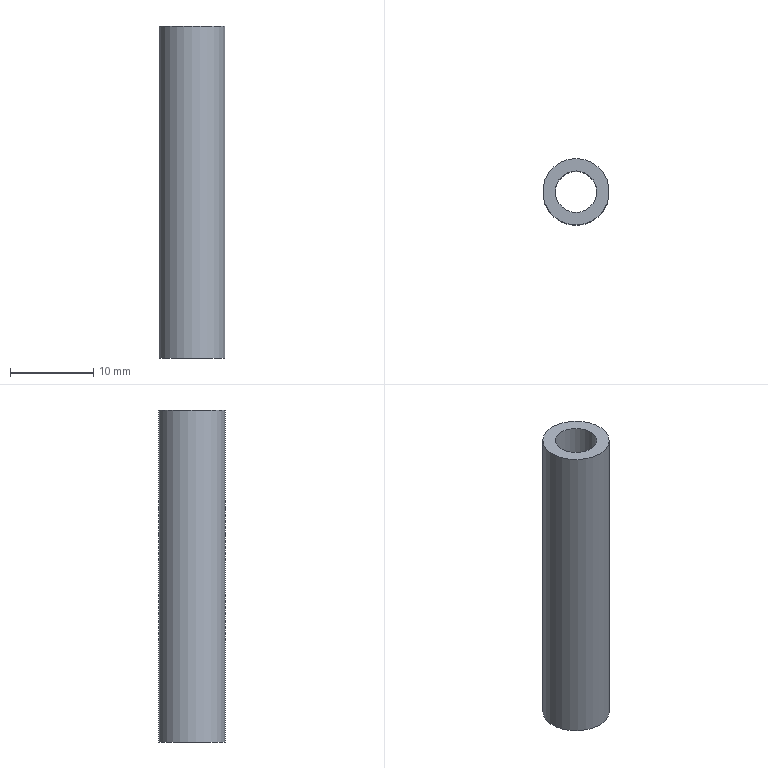Part | STEP file | 1-65.4 | 1 solid | 4 faces | box 8 x 8 x 40 mm | volume 1225 mm3 | plane 2 | cylinder 2 | commonest cylinder face diameters 5 x1 8 x1
STEP:
#1=CARTESIAN_POINT('',(0.,0.,0.));
#2=DIRECTION('',(0.,0.,1.));
#3=DIRECTION('',(1.,0.,0.));
#4=AXIS2_PLACEMENT_3D('',#1,#2,#3);
#5=CARTESIAN_POINT('',(0.,4.,0.));
#6=VERTEX_POINT('',#5);
#7=CARTESIAN_POINT('',(0.,0.,0.));
#8=DIRECTION('',(0.,0.,1.));
#9=DIRECTION('',(0.,1.,0.));
#10=AXIS2_PLACEMENT_3D('',#7,#8,#9);
#11=CIRCLE('',#10,4.);
#12=CARTESIAN_POINT('',(0.,-1.072,0.));
#13=DIRECTION('',(0.,0.,1.));
#14=DIRECTION('',(0.,1.,0.));
#15=AXIS2_PLACEMENT_3D('',#12,#13,#14);
#16=PLANE('',#15);
#17=CARTESIAN_POINT('',(1.072,0.));
#18=DIRECTION('',(1.,0.));
#19=AXIS2_PLACEMENT_2D('',#17,#18);
#20=CIRCLE('',#19,4.);
#21=(GEOMETRIC_REPRESENTATION_CONTEXT(2)PARAMETRIC_REPRESENTATION_CONTEXT()REPRESENTATION_CONTEXT('',''));
#22=DEFINITIONAL_REPRESENTATION('',(#20),#21);
#23=PCURVE('',#16,#22);
#24=CARTESIAN_POINT('',(0.,0.,0.));
#25=DIRECTION('',(0.,0.,1.));
#26=DIRECTION('',(0.,1.,0.));
#27=AXIS2_PLACEMENT_3D('',#24,#25,#26);
#28=CYLINDRICAL_SURFACE('',#27,4.);
#29=CARTESIAN_POINT('',(0.,0.));
#30=DIRECTION('',(1.,0.));
#31=VECTOR('',#30,1.);
#32=LINE('',#29,#31);
#33=(GEOMETRIC_REPRESENTATION_CONTEXT(2)PARAMETRIC_REPRESENTATION_CONTEXT()REPRESENTATION_CONTEXT('',''));
#34=DEFINITIONAL_REPRESENTATION('',(#32),#33);
#35=PCURVE('',#28,#34);
#36=SURFACE_CURVE('',#11,(#23,#35),.PCURVE_S1.);
#37=EDGE_CURVE('',#6,#6,#36,.T.);
#38=ORIENTED_EDGE('',*,*,#37,.T.);
#39=EDGE_LOOP('',(#38));
#40=FACE_BOUND('',#39,.F.);
#41=CARTESIAN_POINT('',(0.,2.5,0.));
#42=VERTEX_POINT('',#41);
#43=CARTESIAN_POINT('',(0.,0.,0.));
#44=DIRECTION('',(0.,0.,-1.));
#45=DIRECTION('',(0.,1.,0.));
#46=AXIS2_PLACEMENT_3D('',#43,#44,#45);
#47=CIRCLE('',#46,2.5);
#48=CARTESIAN_POINT('',(3.572,0.));
#49=CARTESIAN_POINT('',(3.572,-4.33));
#50=CARTESIAN_POINT('',(-0.1782,-2.165));
#51=CARTESIAN_POINT('',(-3.928,0.));
#52=CARTESIAN_POINT('',(-0.1782,2.165));
#53=CARTESIAN_POINT('',(3.572,4.33));
#54=CARTESIAN_POINT('',(3.572,0.));
#55=(BOUNDED_CURVE()B_SPLINE_CURVE(2,(#48,#49,#50,#51,#52,#53,#54),.UNSPECIFIED.,.T.,.F.)B_SPLINE_CURVE_WITH_KNOTS((1,2,2,2,2,1),(-2.094,0.,2.094,4.189,6.283,8.378),.UNSPECIFIED.)CURVE()GEOMETRIC_REPRESENTATION_ITEM()RATIONAL_B_SPLINE_CURVE((1.,0.5,1.,0.5,1.,0.5,1.))REPRESENTATION_ITEM(''));
#56=(GEOMETRIC_REPRESENTATION_CONTEXT(2)PARAMETRIC_REPRESENTATION_CONTEXT()REPRESENTATION_CONTEXT('',''));
#57=DEFINITIONAL_REPRESENTATION('',(#55),#56);
#58=PCURVE('',#16,#57);
#59=CARTESIAN_POINT('',(0.,0.,0.));
#60=DIRECTION('',(0.,0.,1.));
#61=DIRECTION('',(0.,1.,0.));
#62=AXIS2_PLACEMENT_3D('',#59,#60,#61);
#63=CYLINDRICAL_SURFACE('',#62,2.5);
#64=CARTESIAN_POINT('',(6.283,0.));
#65=DIRECTION('',(-1.,0.));
#66=VECTOR('',#65,1.);
#67=LINE('',#64,#66);
#68=(GEOMETRIC_REPRESENTATION_CONTEXT(2)PARAMETRIC_REPRESENTATION_CONTEXT()REPRESENTATION_CONTEXT('',''));
#69=DEFINITIONAL_REPRESENTATION('',(#67),#68);
#70=PCURVE('',#63,#69);
#71=SURFACE_CURVE('',#47,(#58,#70),.PCURVE_S1.);
#72=EDGE_CURVE('',#42,#42,#71,.T.);
#73=ORIENTED_EDGE('',*,*,#72,.T.);
#74=EDGE_LOOP('',(#73));
#75=FACE_BOUND('',#74,.F.);
#76=ADVANCED_FACE('',(#40,#75),#16,.F.);
#77=CARTESIAN_POINT('',(0.,4.,40.));
#78=VERTEX_POINT('',#77);
#79=CARTESIAN_POINT('',(0.,0.,40.));
#80=DIRECTION('',(0.,0.,1.));
#81=DIRECTION('',(0.,1.,0.));
#82=AXIS2_PLACEMENT_3D('',#79,#80,#81);
#83=CIRCLE('',#82,4.);
#84=CARTESIAN_POINT('',(0.,-1.072,40.));
#85=DIRECTION('',(0.,0.,1.));
#86=DIRECTION('',(0.,1.,0.));
#87=AXIS2_PLACEMENT_3D('',#84,#85,#86);
#88=PLANE('',#87);
#89=CARTESIAN_POINT('',(1.072,0.));
#90=DIRECTION('',(1.,0.));
#91=AXIS2_PLACEMENT_2D('',#89,#90);
#92=CIRCLE('',#91,4.);
#93=(GEOMETRIC_REPRESENTATION_CONTEXT(2)PARAMETRIC_REPRESENTATION_CONTEXT()REPRESENTATION_CONTEXT('',''));
#94=DEFINITIONAL_REPRESENTATION('',(#92),#93);
#95=PCURVE('',#88,#94);
#96=CARTESIAN_POINT('',(0.,40.));
#97=DIRECTION('',(1.,0.));
#98=VECTOR('',#97,1.);
#99=LINE('',#96,#98);
#100=(GEOMETRIC_REPRESENTATION_CONTEXT(2)PARAMETRIC_REPRESENTATION_CONTEXT()REPRESENTATION_CONTEXT('',''));
#101=DEFINITIONAL_REPRESENTATION('',(#99),#100);
#102=PCURVE('',#28,#101);
#103=SURFACE_CURVE('',#83,(#95,#102),.PCURVE_S1.);
#104=EDGE_CURVE('',#78,#78,#103,.T.);
#105=ORIENTED_EDGE('',*,*,#104,.T.);
#106=EDGE_LOOP('',(#105));
#107=FACE_BOUND('',#106,.T.);
#108=CARTESIAN_POINT('',(0.,2.5,40.));
#109=VERTEX_POINT('',#108);
#110=CARTESIAN_POINT('',(0.,0.,40.));
#111=DIRECTION('',(0.,0.,-1.));
#112=DIRECTION('',(0.,1.,0.));
#113=AXIS2_PLACEMENT_3D('',#110,#111,#112);
#114=CIRCLE('',#113,2.5);
#115=CARTESIAN_POINT('',(3.572,0.));
#116=CARTESIAN_POINT('',(3.572,-4.33));
#117=CARTESIAN_POINT('',(-0.1782,-2.165));
#118=CARTESIAN_POINT('',(-3.928,0.));
#119=CARTESIAN_POINT('',(-0.1782,2.165));
#120=CARTESIAN_POINT('',(3.572,4.33));
#121=CARTESIAN_POINT('',(3.572,0.));
#122=(BOUNDED_CURVE()B_SPLINE_CURVE(2,(#115,#116,#117,#118,#119,#120,#121),.UNSPECIFIED.,.T.,.F.)B_SPLINE_CURVE_WITH_KNOTS((1,2,2,2,2,1),(-2.094,0.,2.094,4.189,6.283,8.378),.UNSPECIFIED.)CURVE()GEOMETRIC_REPRESENTATION_ITEM()RATIONAL_B_SPLINE_CURVE((1.,0.5,1.,0.5,1.,0.5,1.))REPRESENTATION_ITEM(''));
#123=(GEOMETRIC_REPRESENTATION_CONTEXT(2)PARAMETRIC_REPRESENTATION_CONTEXT()REPRESENTATION_CONTEXT('',''));
#124=DEFINITIONAL_REPRESENTATION('',(#122),#123);
#125=PCURVE('',#88,#124);
#126=CARTESIAN_POINT('',(6.283,40.));
#127=DIRECTION('',(-1.,0.));
#128=VECTOR('',#127,1.);
#129=LINE('',#126,#128);
#130=(GEOMETRIC_REPRESENTATION_CONTEXT(2)PARAMETRIC_REPRESENTATION_CONTEXT()REPRESENTATION_CONTEXT('',''));
#131=DEFINITIONAL_REPRESENTATION('',(#129),#130);
#132=PCURVE('',#63,#131);
#133=SURFACE_CURVE('',#114,(#125,#132),.PCURVE_S1.);
#134=EDGE_CURVE('',#109,#109,#133,.T.);
#135=ORIENTED_EDGE('',*,*,#134,.T.);
#136=EDGE_LOOP('',(#135));
#137=FACE_BOUND('',#136,.T.);
#138=ADVANCED_FACE('',(#107,#137),#88,.T.);
#139=ORIENTED_EDGE('',*,*,#37,.T.);
#140=CARTESIAN_POINT('',(0.,4.,0.));
#141=DIRECTION('',(0.,0.,1.));
#142=VECTOR('',#141,1.);
#143=LINE('',#140,#142);
#144=CARTESIAN_POINT('',(6.283,0.));
#145=DIRECTION('',(0.,1.));
#146=VECTOR('',#145,1.);
#147=LINE('',#144,#146);
#148=(GEOMETRIC_REPRESENTATION_CONTEXT(2)PARAMETRIC_REPRESENTATION_CONTEXT()REPRESENTATION_CONTEXT('',''));
#149=DEFINITIONAL_REPRESENTATION('',(#147),#148);
#150=PCURVE('',#28,#149);
#151=CARTESIAN_POINT('',(0.,0.));
#152=DIRECTION('',(0.,1.));
#153=VECTOR('',#152,1.);
#154=LINE('',#151,#153);
#155=(GEOMETRIC_REPRESENTATION_CONTEXT(2)PARAMETRIC_REPRESENTATION_CONTEXT()REPRESENTATION_CONTEXT('',''));
#156=DEFINITIONAL_REPRESENTATION('',(#154),#155);
#157=PCURVE('',#28,#156);
#158=SEAM_CURVE('',#143,(#150,#157),.PCURVE_S1.);
#159=EDGE_CURVE('',#6,#78,#158,.T.);
#160=ORIENTED_EDGE('',*,*,#159,.T.);
#161=ORIENTED_EDGE('',*,*,#104,.F.);
#162=ORIENTED_EDGE('',*,*,#159,.F.);
#163=EDGE_LOOP('',(#139,#160,#161,#162));
#164=FACE_BOUND('',#163,.T.);
#165=ADVANCED_FACE('',(#164),#28,.T.);
#166=CARTESIAN_POINT('',(0.,2.5,0.));
#167=DIRECTION('',(0.,0.,1.));
#168=VECTOR('',#167,1.);
#169=LINE('',#166,#168);
#170=CARTESIAN_POINT('',(6.283,0.));
#171=DIRECTION('',(0.,1.));
#172=VECTOR('',#171,1.);
#173=LINE('',#170,#172);
#174=(GEOMETRIC_REPRESENTATION_CONTEXT(2)PARAMETRIC_REPRESENTATION_CONTEXT()REPRESENTATION_CONTEXT('',''));
#175=DEFINITIONAL_REPRESENTATION('',(#173),#174);
#176=PCURVE('',#63,#175);
#177=CARTESIAN_POINT('',(0.,0.));
#178=DIRECTION('',(0.,1.));
#179=VECTOR('',#178,1.);
#180=LINE('',#177,#179);
#181=(GEOMETRIC_REPRESENTATION_CONTEXT(2)PARAMETRIC_REPRESENTATION_CONTEXT()REPRESENTATION_CONTEXT('',''));
#182=DEFINITIONAL_REPRESENTATION('',(#180),#181);
#183=PCURVE('',#63,#182);
#184=SEAM_CURVE('',#169,(#176,#183),.PCURVE_S1.);
#185=EDGE_CURVE('',#42,#109,#184,.T.);
#186=ORIENTED_EDGE('',*,*,#185,.T.);
#187=ORIENTED_EDGE('',*,*,#134,.T.);
#188=ORIENTED_EDGE('',*,*,#185,.F.);
#189=ORIENTED_EDGE('',*,*,#72,.F.);
#190=EDGE_LOOP('',(#186,#187,#188,#189));
#191=FACE_BOUND('',#190,.F.);
#192=ADVANCED_FACE('',(#191),#63,.F.);
#193=CLOSED_SHELL('',(#76,#138,#165,#192));
#194=MANIFOLD_SOLID_BREP('',#193);
#195=(LENGTH_UNIT()NAMED_UNIT(*)SI_UNIT(.MILLI.,.METRE.));
#196=UNCERTAINTY_MEASURE_WITH_UNIT(LENGTH_MEASURE(0.0000001),#195,'','');
#197=(NAMED_UNIT(*)PLANE_ANGLE_UNIT()SI_UNIT($,.RADIAN.));
#198=(NAMED_UNIT(*)SI_UNIT($,.STERADIAN.)SOLID_ANGLE_UNIT());
#199=(GEOMETRIC_REPRESENTATION_CONTEXT(3)GLOBAL_UNCERTAINTY_ASSIGNED_CONTEXT((#196))GLOBAL_UNIT_ASSIGNED_CONTEXT((#195,#197,#198))REPRESENTATION_CONTEXT('',''));
#200=ADVANCED_BREP_SHAPE_REPRESENTATION('',(#4,#194),#199);